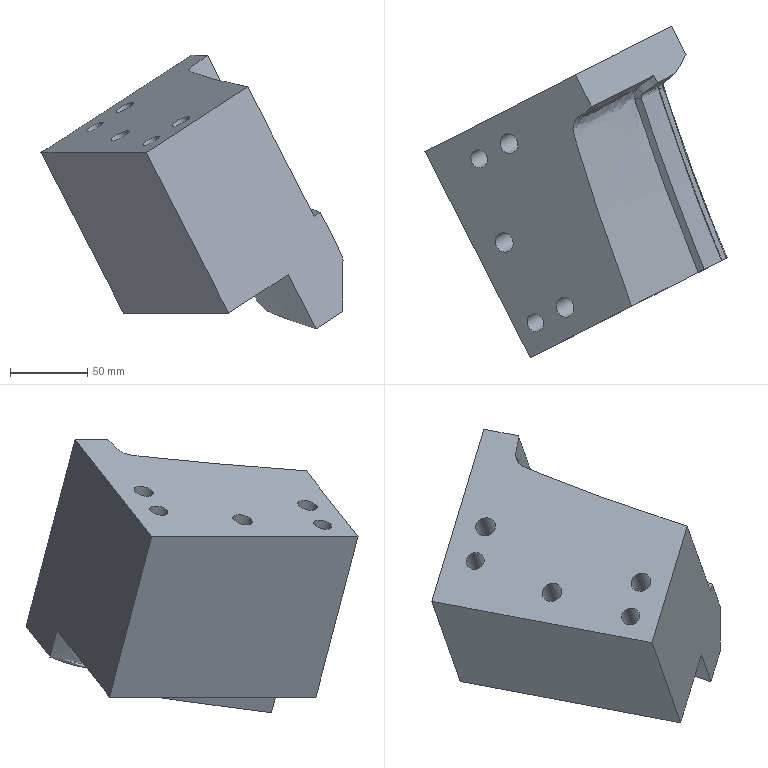Part | NX | features solid 2 | 1 solid | 45 faces | box 195.611 x 215.025 x 177.136 mm | volume 1843071 mm3 | spline 23 | plane 12 | cylinder 10 | commonest cylinder face diameters 13 x3 20 x3 12 x2 14 x2